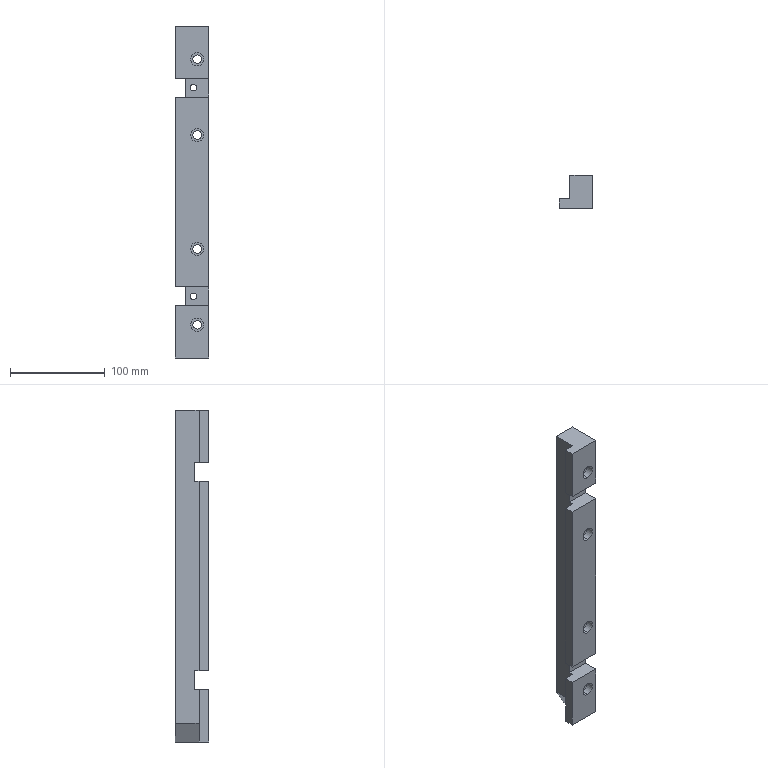Part | STEP file | OP10-021_guide(1) | 1 solid | 45 faces | box 35 x 35 x 350 mm | volume 297564 mm3 | plane 25 | cylinder 20 | commonest cylinder face diameters 9 x8 14 x8 6.8 x4